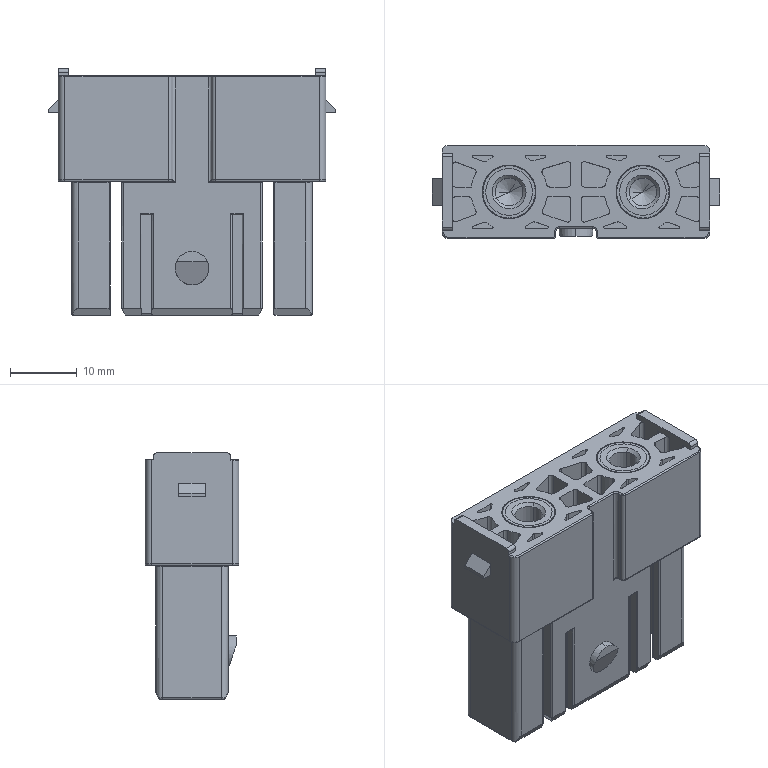Part | NX | features BREP 2 | 3 solids | 1907 faces | box 43 x 14 x 36.8 mm | volume 9836 mm3 | plane 1136 | cylinder 705 | torus 38 | sphere 14 | cone 8 | spline 6 | commonest cylinder face diameters 8 x498 0.4 x118 1 x51 11.4 x16 2 x8 7 x8